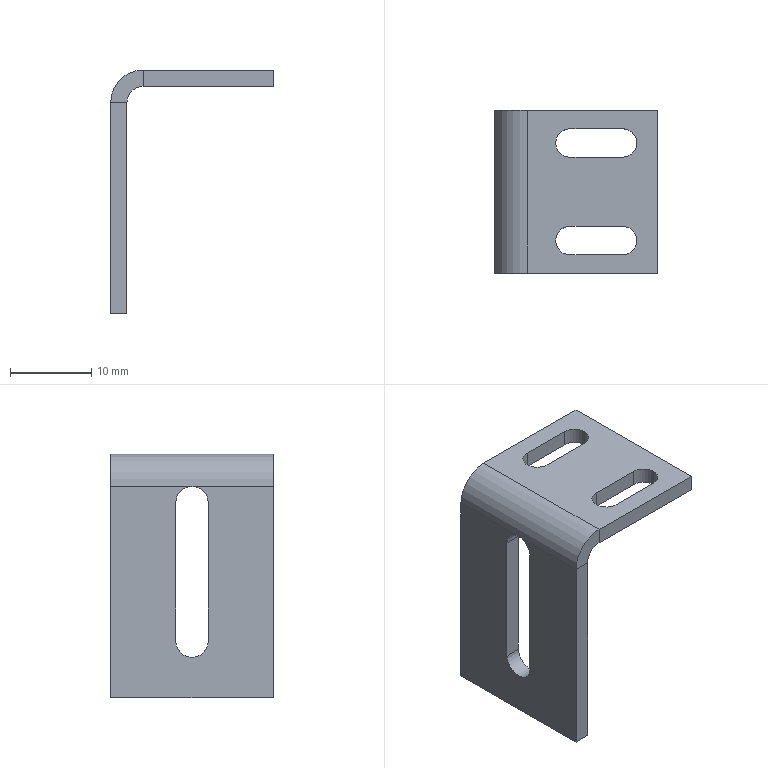Part | STEP file | M12 laser diffuse reflection sensor bracket 1001 | 1 solid | 29 faces | box 20 x 20 x 30 mm | volume 1578 mm3 | plane 18 | cylinder 11 | commonest cylinder face diameters 3.5 x6 4 x4 8 x1